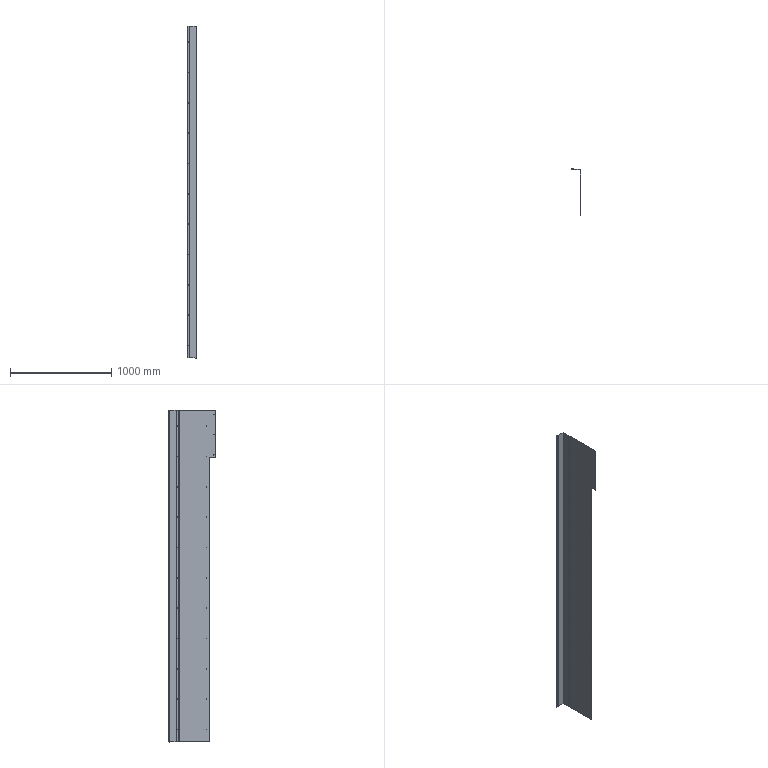Part | STEP file | TS-S32 | 1 solid | 136 faces | box 95.999 x 457.999 x 3283 mm | volume 1963337 mm3 | cylinder 86 | plane 50 | commonest cylinder face diameters 5.4 x72 0.4 x7 2.8 x7